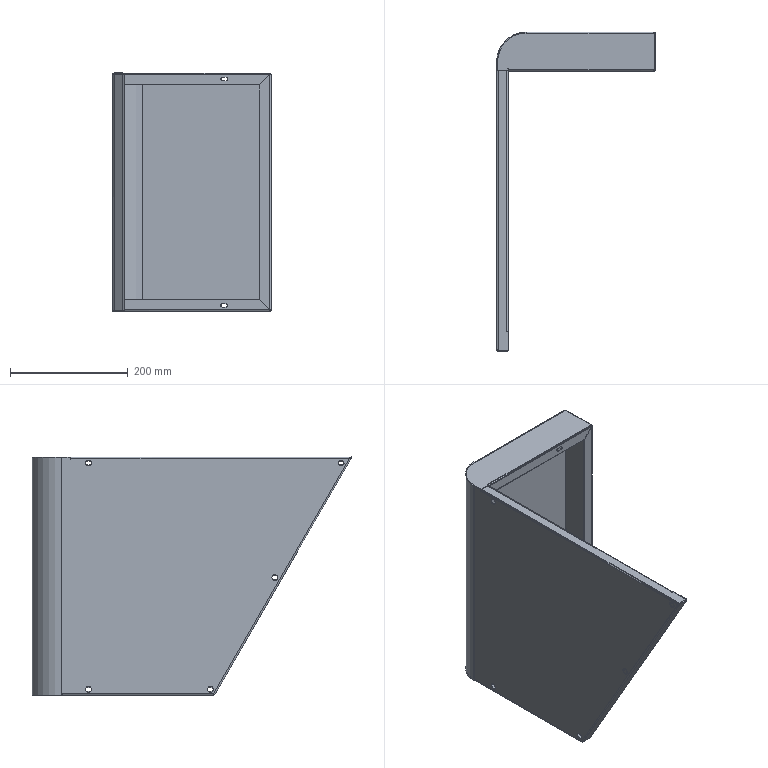Part | SolidWorks | features MirrorStock 1 | 1 solid | 218 faces | box 270 x 544 x 405.75 mm | volume 580756 mm3 | plane 144 | cylinder 64 | spline 10 | commonest cylinder face diameters 6 x21 10 x14 2 x12 5 x12 96.6 x3 97 x1